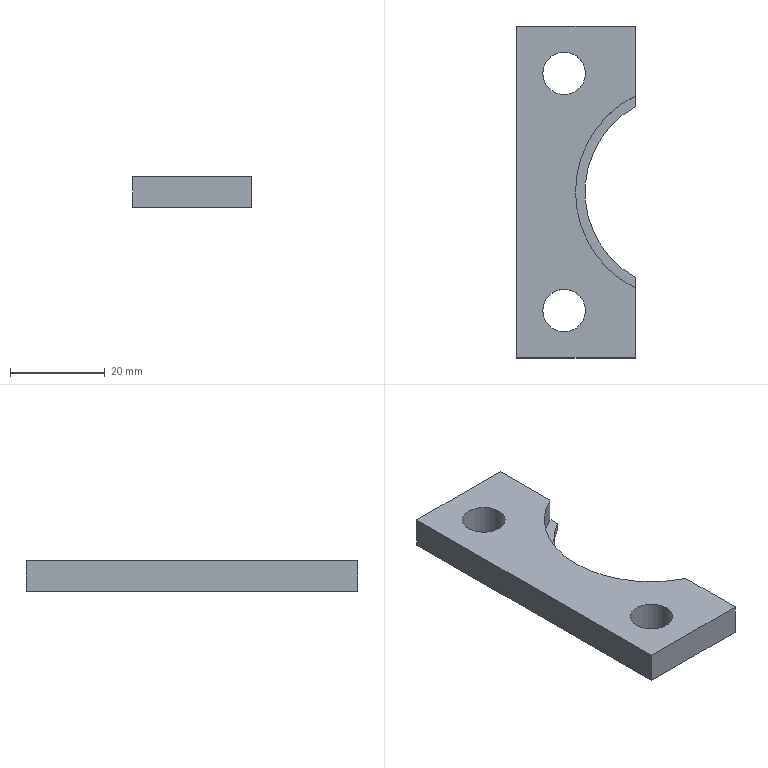Part | NX | features solid 2 | 1 solid | 12 faces | box 25 x 70 x 6.5 mm | volume 8313 mm3 | plane 8 | cylinder 4 | commonest cylinder face diameters 9 x2 41.2 x1 45.2 x1
STEP:
#1=CARTESIAN_POINT('',(-1170.,-560.,17.));
#2=VERTEX_POINT('',#1);
#3=CARTESIAN_POINT('',(-1170.,-574.733,17.));
#4=VERTEX_POINT('',#3);
#5=CARTESIAN_POINT('',(-1170.,-560.,17.));
#6=DIRECTION('',(0.,-1.,0.));
#7=VECTOR('',#6,1000.);
#8=LINE('',#5,#7);
#9=EDGE_CURVE('',#2,#4,#8,.T.);
#10=ORIENTED_EDGE('',*,*,#9,.F.);
#11=CARTESIAN_POINT('',(-1195.,-560.,17.));
#12=VERTEX_POINT('',#11);
#13=CARTESIAN_POINT('',(-1160.,-560.,17.));
#14=DIRECTION('',(1.,0.,0.));
#15=VECTOR('',#14,1000.);
#16=LINE('',#13,#15);
#17=EDGE_CURVE('',#12,#2,#16,.T.);
#18=ORIENTED_EDGE('',*,*,#17,.F.);
#19=CARTESIAN_POINT('',(-1195.,-630.,17.));
#20=VERTEX_POINT('',#19);
#21=CARTESIAN_POINT('',(-1195.,-560.,17.));
#22=DIRECTION('',(0.,1.,0.));
#23=VECTOR('',#22,1000.);
#24=LINE('',#21,#23);
#25=EDGE_CURVE('',#12,#20,#24,.F.);
#26=ORIENTED_EDGE('',*,*,#25,.T.);
#27=CARTESIAN_POINT('',(-1170.,-630.,17.));
#28=VERTEX_POINT('',#27);
#29=CARTESIAN_POINT('',(-1160.,-630.,17.));
#30=DIRECTION('',(1.,0.,0.));
#31=VECTOR('',#30,1000.);
#32=LINE('',#29,#31);
#33=EDGE_CURVE('',#20,#28,#32,.T.);
#34=ORIENTED_EDGE('',*,*,#33,.T.);
#35=CARTESIAN_POINT('',(-1170.,-615.267,17.));
#36=VERTEX_POINT('',#35);
#37=CARTESIAN_POINT('',(-1170.,-560.,17.));
#38=DIRECTION('',(0.,-1.,0.));
#39=VECTOR('',#38,1000.);
#40=LINE('',#37,#39);
#41=EDGE_CURVE('',#36,#28,#40,.T.);
#42=ORIENTED_EDGE('',*,*,#41,.F.);
#43=CARTESIAN_POINT('',(-1160.,-595.,17.));
#44=DIRECTION('',(0.,0.,-1.));
#45=DIRECTION('',(-1.,0.,0.));
#46=AXIS2_PLACEMENT_3D('',#43,#44,#45);
#47=CIRCLE('',#46,22.6);
#48=EDGE_CURVE('',#36,#4,#47,.T.);
#49=ORIENTED_EDGE('',*,*,#48,.T.);
#50=EDGE_LOOP('',(#10,#18,#26,#34,#42,#49));
#51=FACE_BOUND('',#50,.T.);
#52=CARTESIAN_POINT('',(-1180.5,-570.,17.));
#53=VERTEX_POINT('',#52);
#54=CARTESIAN_POINT('',(-1185.,-570.,17.));
#55=DIRECTION('',(0.,0.,1.));
#56=DIRECTION('',(1.,0.,0.));
#57=AXIS2_PLACEMENT_3D('',#54,#55,#56);
#58=CIRCLE('',#57,4.5);
#59=EDGE_CURVE('',#53,#53,#58,.T.);
#60=ORIENTED_EDGE('',*,*,#59,.F.);
#61=EDGE_LOOP('',(#60));
#62=FACE_BOUND('',#61,.T.);
#63=CARTESIAN_POINT('',(-1180.5,-620.,17.));
#64=VERTEX_POINT('',#63);
#65=CARTESIAN_POINT('',(-1185.,-620.,17.));
#66=DIRECTION('',(0.,0.,1.));
#67=DIRECTION('',(1.,0.,0.));
#68=AXIS2_PLACEMENT_3D('',#65,#66,#67);
#69=CIRCLE('',#68,4.5);
#70=EDGE_CURVE('',#64,#64,#69,.T.);
#71=ORIENTED_EDGE('',*,*,#70,.F.);
#72=EDGE_LOOP('',(#71));
#73=FACE_BOUND('',#72,.T.);
#74=CARTESIAN_POINT('',(-1160.,-560.,17.));
#75=DIRECTION('',(0.,0.,1.));
#76=DIRECTION('',(0.,-1.,0.));
#77=AXIS2_PLACEMENT_3D('',#74,#75,#76);
#78=PLANE('',#77);
#79=ADVANCED_FACE('',(#51,#62,#73),#78,.T.);
#80=CARTESIAN_POINT('',(-1170.,-630.,10.5));
#81=VERTEX_POINT('',#80);
#82=CARTESIAN_POINT('',(-1170.,-630.,17.));
#83=DIRECTION('',(0.,0.,-1.));
#84=VECTOR('',#83,1000.);
#85=LINE('',#82,#84);
#86=EDGE_CURVE('',#28,#81,#85,.T.);
#87=ORIENTED_EDGE('',*,*,#86,.F.);
#88=ORIENTED_EDGE('',*,*,#33,.F.);
#89=CARTESIAN_POINT('',(-1195.,-630.,10.5));
#90=VERTEX_POINT('',#89);
#91=CARTESIAN_POINT('',(-1195.,-630.,17.));
#92=DIRECTION('',(0.,0.,-1.));
#93=VECTOR('',#92,1000.);
#94=LINE('',#91,#93);
#95=EDGE_CURVE('',#20,#90,#94,.T.);
#96=ORIENTED_EDGE('',*,*,#95,.T.);
#97=CARTESIAN_POINT('',(-1160.,-630.,10.5));
#98=DIRECTION('',(1.,0.,0.));
#99=VECTOR('',#98,1000.);
#100=LINE('',#97,#99);
#101=EDGE_CURVE('',#90,#81,#100,.T.);
#102=ORIENTED_EDGE('',*,*,#101,.T.);
#103=EDGE_LOOP('',(#87,#88,#96,#102));
#104=FACE_BOUND('',#103,.T.);
#105=CARTESIAN_POINT('',(-1160.,-630.,17.));
#106=DIRECTION('',(0.,-1.,0.));
#107=DIRECTION('',(0.,0.,-1.));
#108=AXIS2_PLACEMENT_3D('',#105,#106,#107);
#109=PLANE('',#108);
#110=ADVANCED_FACE('',(#104),#109,.T.);
#111=CARTESIAN_POINT('',(-1170.,-613.01,10.5));
#112=VERTEX_POINT('',#111);
#113=CARTESIAN_POINT('',(-1170.,-560.,10.5));
#114=DIRECTION('',(0.,-1.,0.));
#115=VECTOR('',#114,1000.);
#116=LINE('',#113,#115);
#117=EDGE_CURVE('',#81,#112,#116,.F.);
#118=ORIENTED_EDGE('',*,*,#117,.F.);
#119=ORIENTED_EDGE('',*,*,#101,.F.);
#120=CARTESIAN_POINT('',(-1195.,-560.,10.5));
#121=VERTEX_POINT('',#120);
#122=CARTESIAN_POINT('',(-1195.,-560.,10.5));
#123=DIRECTION('',(0.,1.,0.));
#124=VECTOR('',#123,1000.);
#125=LINE('',#122,#124);
#126=EDGE_CURVE('',#121,#90,#125,.F.);
#127=ORIENTED_EDGE('',*,*,#126,.F.);
#128=CARTESIAN_POINT('',(-1170.,-560.,10.5));
#129=VERTEX_POINT('',#128);
#130=CARTESIAN_POINT('',(-1160.,-560.,10.5));
#131=DIRECTION('',(1.,0.,0.));
#132=VECTOR('',#131,1000.);
#133=LINE('',#130,#132);
#134=EDGE_CURVE('',#121,#129,#133,.T.);
#135=ORIENTED_EDGE('',*,*,#134,.T.);
#136=CARTESIAN_POINT('',(-1170.,-576.99,10.5));
#137=VERTEX_POINT('',#136);
#138=CARTESIAN_POINT('',(-1170.,-560.,10.5));
#139=DIRECTION('',(0.,-1.,0.));
#140=VECTOR('',#139,1000.);
#141=LINE('',#138,#140);
#142=EDGE_CURVE('',#137,#129,#141,.F.);
#143=ORIENTED_EDGE('',*,*,#142,.F.);
#144=CARTESIAN_POINT('',(-1160.,-595.,10.5));
#145=DIRECTION('',(0.,0.,1.));
#146=DIRECTION('',(1.,0.,0.));
#147=AXIS2_PLACEMENT_3D('',#144,#145,#146);
#148=CIRCLE('',#147,20.6);
#149=EDGE_CURVE('',#112,#137,#148,.F.);
#150=ORIENTED_EDGE('',*,*,#149,.F.);
#151=EDGE_LOOP('',(#118,#119,#127,#135,#143,#150));
#152=FACE_BOUND('',#151,.T.);
#153=CARTESIAN_POINT('',(-1180.5,-570.,10.5));
#154=VERTEX_POINT('',#153);
#155=CARTESIAN_POINT('',(-1185.,-570.,10.5));
#156=DIRECTION('',(0.,0.,1.));
#157=DIRECTION('',(1.,0.,0.));
#158=AXIS2_PLACEMENT_3D('',#155,#156,#157);
#159=CIRCLE('',#158,4.5);
#160=EDGE_CURVE('',#154,#154,#159,.T.);
#161=ORIENTED_EDGE('',*,*,#160,.T.);
#162=EDGE_LOOP('',(#161));
#163=FACE_BOUND('',#162,.T.);
#164=CARTESIAN_POINT('',(-1180.5,-620.,10.5));
#165=VERTEX_POINT('',#164);
#166=CARTESIAN_POINT('',(-1185.,-620.,10.5));
#167=DIRECTION('',(0.,0.,1.));
#168=DIRECTION('',(1.,0.,0.));
#169=AXIS2_PLACEMENT_3D('',#166,#167,#168);
#170=CIRCLE('',#169,4.5);
#171=EDGE_CURVE('',#165,#165,#170,.T.);
#172=ORIENTED_EDGE('',*,*,#171,.T.);
#173=EDGE_LOOP('',(#172));
#174=FACE_BOUND('',#173,.T.);
#175=CARTESIAN_POINT('',(-1160.,-560.,10.5));
#176=DIRECTION('',(0.,0.,1.));
#177=DIRECTION('',(0.,-1.,0.));
#178=AXIS2_PLACEMENT_3D('',#175,#176,#177);
#179=PLANE('',#178);
#180=ADVANCED_FACE('',(#152,#163,#174),#179,.F.);
#181=CARTESIAN_POINT('',(-1170.,-560.,17.));
#182=DIRECTION('',(0.,0.,-1.));
#183=VECTOR('',#182,1000.);
#184=LINE('',#181,#183);
#185=EDGE_CURVE('',#129,#2,#184,.F.);
#186=ORIENTED_EDGE('',*,*,#185,.F.);
#187=ORIENTED_EDGE('',*,*,#134,.F.);
#188=CARTESIAN_POINT('',(-1195.,-560.,17.));
#189=DIRECTION('',(0.,0.,-1.));
#190=VECTOR('',#189,1000.);
#191=LINE('',#188,#190);
#192=EDGE_CURVE('',#12,#121,#191,.T.);
#193=ORIENTED_EDGE('',*,*,#192,.F.);
#194=ORIENTED_EDGE('',*,*,#17,.T.);
#195=EDGE_LOOP('',(#186,#187,#193,#194));
#196=FACE_BOUND('',#195,.T.);
#197=CARTESIAN_POINT('',(-1160.,-560.,17.));
#198=DIRECTION('',(0.,-1.,0.));
#199=DIRECTION('',(0.,0.,-1.));
#200=AXIS2_PLACEMENT_3D('',#197,#198,#199);
#201=PLANE('',#200);
#202=ADVANCED_FACE('',(#196),#201,.F.);
#203=ORIENTED_EDGE('',*,*,#126,.T.);
#204=ORIENTED_EDGE('',*,*,#95,.F.);
#205=ORIENTED_EDGE('',*,*,#25,.F.);
#206=ORIENTED_EDGE('',*,*,#192,.T.);
#207=EDGE_LOOP('',(#203,#204,#205,#206));
#208=FACE_BOUND('',#207,.T.);
#209=CARTESIAN_POINT('',(-1195.,-560.,17.));
#210=DIRECTION('',(1.,0.,0.));
#211=DIRECTION('',(0.,0.,-1.));
#212=AXIS2_PLACEMENT_3D('',#209,#210,#211);
#213=PLANE('',#212);
#214=ADVANCED_FACE('',(#208),#213,.F.);
#215=ORIENTED_EDGE('',*,*,#149,.T.);
#216=CARTESIAN_POINT('',(-1170.,-576.99,12.));
#217=VERTEX_POINT('',#216);
#218=CARTESIAN_POINT('',(-1170.,-576.99,13.));
#219=DIRECTION('',(0.,0.,-1.));
#220=VECTOR('',#219,1000.);
#221=LINE('',#218,#220);
#222=EDGE_CURVE('',#137,#217,#221,.F.);
#223=ORIENTED_EDGE('',*,*,#222,.T.);
#224=CARTESIAN_POINT('',(-1170.,-613.01,12.));
#225=VERTEX_POINT('',#224);
#226=CARTESIAN_POINT('',(-1160.,-595.,12.));
#227=DIRECTION('',(0.,0.,1.));
#228=DIRECTION('',(1.,0.,0.));
#229=AXIS2_PLACEMENT_3D('',#226,#227,#228);
#230=CIRCLE('',#229,20.6);
#231=EDGE_CURVE('',#225,#217,#230,.F.);
#232=ORIENTED_EDGE('',*,*,#231,.F.);
#233=CARTESIAN_POINT('',(-1170.,-613.01,13.));
#234=DIRECTION('',(0.,0.,-1.));
#235=VECTOR('',#234,1000.);
#236=LINE('',#233,#235);
#237=EDGE_CURVE('',#225,#112,#236,.T.);
#238=ORIENTED_EDGE('',*,*,#237,.T.);
#239=EDGE_LOOP('',(#215,#223,#232,#238));
#240=FACE_BOUND('',#239,.T.);
#241=CARTESIAN_POINT('',(-1160.,-595.,13.));
#242=DIRECTION('',(0.,0.,-1.));
#243=DIRECTION('',(-1.,0.,0.));
#244=AXIS2_PLACEMENT_3D('',#241,#242,#243);
#245=CYLINDRICAL_SURFACE('',#244,20.6);
#246=ADVANCED_FACE('',(#240),#245,.F.);
#247=CARTESIAN_POINT('',(-1170.,-574.733,12.));
#248=VERTEX_POINT('',#247);
#249=CARTESIAN_POINT('',(-1170.,-574.733,13.));
#250=DIRECTION('',(0.,0.,1.));
#251=VECTOR('',#250,1000.);
#252=LINE('',#249,#251);
#253=EDGE_CURVE('',#248,#4,#252,.T.);
#254=ORIENTED_EDGE('',*,*,#253,.T.);
#255=ORIENTED_EDGE('',*,*,#48,.F.);
#256=CARTESIAN_POINT('',(-1170.,-615.267,12.));
#257=VERTEX_POINT('',#256);
#258=CARTESIAN_POINT('',(-1170.,-615.267,-63.));
#259=DIRECTION('',(0.,0.,1.));
#260=VECTOR('',#259,1000.);
#261=LINE('',#258,#260);
#262=EDGE_CURVE('',#36,#257,#261,.F.);
#263=ORIENTED_EDGE('',*,*,#262,.T.);
#264=CARTESIAN_POINT('',(-1160.,-595.,12.));
#265=DIRECTION('',(0.,0.,-1.));
#266=DIRECTION('',(-1.,0.,0.));
#267=AXIS2_PLACEMENT_3D('',#264,#265,#266);
#268=CIRCLE('',#267,22.6);
#269=EDGE_CURVE('',#257,#248,#268,.T.);
#270=ORIENTED_EDGE('',*,*,#269,.T.);
#271=EDGE_LOOP('',(#254,#255,#263,#270));
#272=FACE_BOUND('',#271,.T.);
#273=CARTESIAN_POINT('',(-1160.,-595.,-63.));
#274=DIRECTION('',(0.,0.,1.));
#275=DIRECTION('',(1.,0.,0.));
#276=AXIS2_PLACEMENT_3D('',#273,#274,#275);
#277=CYLINDRICAL_SURFACE('',#276,22.6);
#278=ADVANCED_FACE('',(#272),#277,.F.);
#279=ORIENTED_EDGE('',*,*,#70,.T.);
#280=EDGE_LOOP('',(#279));
#281=FACE_BOUND('',#280,.T.);
#282=ORIENTED_EDGE('',*,*,#171,.F.);
#283=EDGE_LOOP('',(#282));
#284=FACE_BOUND('',#283,.T.);
#285=CARTESIAN_POINT('',(-1185.,-620.,10.5));
#286=DIRECTION('',(0.,0.,1.));
#287=DIRECTION('',(1.,0.,0.));
#288=AXIS2_PLACEMENT_3D('',#285,#286,#287);
#289=CYLINDRICAL_SURFACE('',#288,4.5);
#290=ADVANCED_FACE('',(#281,#284),#289,.F.);
#291=ORIENTED_EDGE('',*,*,#59,.T.);
#292=EDGE_LOOP('',(#291));
#293=FACE_BOUND('',#292,.T.);
#294=ORIENTED_EDGE('',*,*,#160,.F.);
#295=EDGE_LOOP('',(#294));
#296=FACE_BOUND('',#295,.T.);
#297=CARTESIAN_POINT('',(-1185.,-570.,10.5));
#298=DIRECTION('',(0.,0.,1.));
#299=DIRECTION('',(1.,0.,0.));
#300=AXIS2_PLACEMENT_3D('',#297,#298,#299);
#301=CYLINDRICAL_SURFACE('',#300,4.5);
#302=ADVANCED_FACE('',(#293,#296),#301,.F.);
#303=ORIENTED_EDGE('',*,*,#253,.F.);
#304=CARTESIAN_POINT('',(-1170.,-630.,12.));
#305=DIRECTION('',(0.,-1.,0.));
#306=VECTOR('',#305,1000.);
#307=LINE('',#304,#306);
#308=EDGE_CURVE('',#248,#217,#307,.T.);
#309=ORIENTED_EDGE('',*,*,#308,.T.);
#310=ORIENTED_EDGE('',*,*,#222,.F.);
#311=ORIENTED_EDGE('',*,*,#142,.T.);
#312=ORIENTED_EDGE('',*,*,#185,.T.);
#313=ORIENTED_EDGE('',*,*,#9,.T.);
#314=EDGE_LOOP('',(#303,#309,#310,#311,#312,#313));
#315=FACE_BOUND('',#314,.T.);
#316=CARTESIAN_POINT('',(-1170.,-630.,17.));
#317=DIRECTION('',(-1.,0.,0.));
#318=DIRECTION('',(0.,0.,1.));
#319=AXIS2_PLACEMENT_3D('',#316,#317,#318);
#320=PLANE('',#319);
#321=ADVANCED_FACE('',(#315),#320,.F.);
#322=CARTESIAN_POINT('',(-1170.,-630.,12.));
#323=DIRECTION('',(0.,-1.,0.));
#324=VECTOR('',#323,1000.);
#325=LINE('',#322,#324);
#326=EDGE_CURVE('',#225,#257,#325,.T.);
#327=ORIENTED_EDGE('',*,*,#326,.T.);
#328=ORIENTED_EDGE('',*,*,#262,.F.);
#329=ORIENTED_EDGE('',*,*,#41,.T.);
#330=ORIENTED_EDGE('',*,*,#86,.T.);
#331=ORIENTED_EDGE('',*,*,#117,.T.);
#332=ORIENTED_EDGE('',*,*,#237,.F.);
#333=EDGE_LOOP('',(#327,#328,#329,#330,#331,#332));
#334=FACE_BOUND('',#333,.T.);
#335=CARTESIAN_POINT('',(-1170.,-630.,17.));
#336=DIRECTION('',(-1.,0.,0.));
#337=DIRECTION('',(0.,0.,1.));
#338=AXIS2_PLACEMENT_3D('',#335,#336,#337);
#339=PLANE('',#338);
#340=ADVANCED_FACE('',(#334),#339,.F.);
#341=ORIENTED_EDGE('',*,*,#269,.F.);
#342=ORIENTED_EDGE('',*,*,#326,.F.);
#343=ORIENTED_EDGE('',*,*,#231,.T.);
#344=ORIENTED_EDGE('',*,*,#308,.F.);
#345=EDGE_LOOP('',(#341,#342,#343,#344));
#346=FACE_BOUND('',#345,.T.);
#347=CARTESIAN_POINT('',(-1160.,-595.,12.));
#348=DIRECTION('',(0.,0.,-1.));
#349=DIRECTION('',(-1.,0.,0.));
#350=AXIS2_PLACEMENT_3D('',#347,#348,#349);
#351=PLANE('',#350);
#352=ADVANCED_FACE('',(#346),#351,.F.);
#353=CLOSED_SHELL('',(#79,#110,#180,#202,#214,#246,#278,#290,#302,#321,#340,#352));
#354=MANIFOLD_SOLID_BREP('',#353);
#355=(LENGTH_UNIT()NAMED_UNIT(*)SI_UNIT(.MILLI.,.METRE.));
#356=UNCERTAINTY_MEASURE_WITH_UNIT(LENGTH_MEASURE(0.00001),#355,'','');
#357=(NAMED_UNIT(*)PLANE_ANGLE_UNIT()SI_UNIT($,.RADIAN.));
#358=(NAMED_UNIT(*)SI_UNIT($,.STERADIAN.)SOLID_ANGLE_UNIT());
#359=(GEOMETRIC_REPRESENTATION_CONTEXT(3)GLOBAL_UNCERTAINTY_ASSIGNED_CONTEXT((#356))GLOBAL_UNIT_ASSIGNED_CONTEXT((#355,#357,#358))REPRESENTATION_CONTEXT('',''));
#360=ADVANCED_BREP_SHAPE_REPRESENTATION('',(#354),#359);